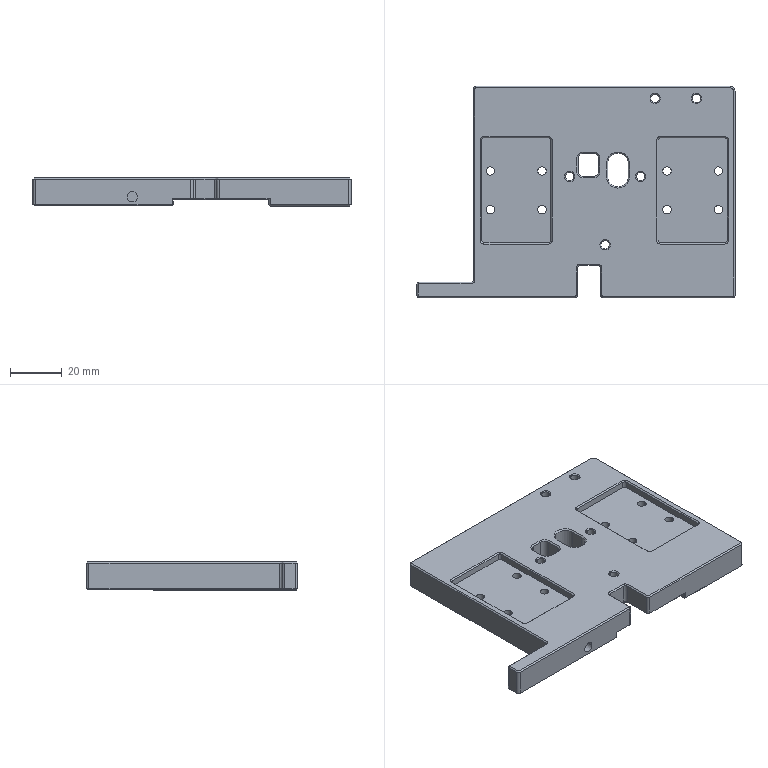NC program | NX | posted with a generic post | part box 123.41 x 82 x 11.078 mm
Whole program:
N10 G17 G21 G94 G90
(ZLEVEL_PROFILE_COPY_COPY_COPY_COPY_COPY_1 , TOOL : D10)
N12 T10 M6
N14 G54
N16 G17 G0 G90 X-32.118 Y-47.254 S9500 M3
N18 G43 Z30. H10
N20 Z4.5
N22 G94 G1 Z3. F1000.
N24 X-32.353 Y-46.848
N26 G3 X-33.219 Y-46.348 R1.
N28 G1 X-38.699 F1200.
N30 X-38.713 Y-46.35
N32 G2 X-45.055 Y-39.992 R6.351
N34 G1 Y29.65
N36 X-60.709
N38 G2 X-62.088 Y29.803 R6.346
N40 G1 X-62.403 Y29.887
N42 G2 X-63.961 Y30.555 R5.799
N44 G1 X-64.243 Y30.729
N46 G2 X-67.055 Y36.009 R6.347
N48 G1 Y39.985
N50 G2 X-66.732 Y41.879 R5.928
N52 X-63.518 Y45.645 R6.354
N54 X-60.764 Y46.31 R6.48
N56 X-55.255 Y46.345 R551.466
N58 G3 X-54.389 Y46.846 R1.
N60 G1 X-54.152 Y47.257
N62 Z4.5
N64 G0 Z30.
N66 X-54.149 Y47.258
N68 Z3.5
N70 G1 Z2. F1000.
N72 X-54.388 Y46.846
N74 G2 X-55.255 Y46.346 R1.
N76 G3 X-60.764 Y46.311 R383.966 F1200.
N78 X-63.977 Y45.394 R6.459
N80 X-65.035 Y44.59 R7.973
N82 X-66.754 Y41.818 R6.483
N84 X-67.055 Y39.985 R5.907
N86 G1 Y36.009
N88 G3 X-64.243 Y30.729 R6.348
N90 G1 X-63.961 Y30.555
N92 G3 X-62.403 Y29.887 R5.803
N94 G1 X-62.088 Y29.803
N96 G3 X-60.709 Y29.65 R6.348
N98 G1 X-45.055
N100 Y-39.992
N102 G3 X-38.713 Y-46.35 R6.351
N104 G1 X-38.699 Y-46.348
N106 X-33.219
N108 G2 X-32.353 Y-46.848 R1.
N110 G1 X-32.118 Y-47.255
N112 Z3.5
N114 G0 Z30.
N116 Z2.5
N118 G1 Z1. F1000.
N120 X-32.353 Y-46.848
N122 G3 X-33.219 Y-46.348 R1.
N124 G1 X-38.699 F1200.
N126 X-38.713 Y-46.35
N128 G2 X-45.055 Y-39.992 R6.351
N130 G1 Y29.65
N132 X-60.709
N134 G2 X-62.089 Y29.803 R6.35
N136 G1 X-62.402 Y29.886
N138 G2 X-63.962 Y30.556 R5.808
N140 G1 X-64.243 Y30.729
N142 G2 X-67.055 Y36.009 R6.348
N144 G1 Y39.985
N146 G2 X-63.977 Y45.4 R6.458
N148 X-60.764 Y46.315 R6.42
N150 X-55.255 Y46.348 R309.642
N152 G3 X-54.387 Y46.845 R1.
N154 G1 X-54.146 Y47.259
N156 Z2.5
N158 G0 Z30.
N160 X-54.153 Y47.261
N162 Z1.5
N164 G1 Z0. F1000.
N166 X-54.39 Y46.849
N168 G2 X-55.255 Y46.348 R1.
N170 G1 X-60.764 Y46.336 F1200.
N172 G3 X-63.518 Y45.676 R6.465
N174 X-67.055 Y39.985 R6.391
N176 G1 Y36.009
N178 G3 X-64.243 Y30.729 R6.348
N180 G1 X-63.962 Y30.556
N182 G3 X-62.402 Y29.886 R5.812
N184 G1 X-62.089 Y29.803
N186 G3 X-60.709 Y29.65 R6.364
N188 G1 X-45.055
N190 Y-39.992
N192 G3 X-38.713 Y-46.35 R6.351
N194 G1 X-38.699 Y-46.348
N196 X-33.219
N198 G2 X-32.353 Y-46.848 R1.
N200 G1 X-32.118 Y-47.255
N202 Z1.5
N204 G0 Z30.
N206 X-32.063 Y-47.35
N208 Z0.5
N210 G1 Z-1. F1000.
N212 X-32.353 Y-46.848
N214 G3 X-33.219 Y-46.348 R1.
N216 G1 X-38.269 F1200.
N218 X-38.705 Y-46.35
N220 G2 X-45.055 Y-40. R6.35
N222 G1 Y29.65
N224 X-60.701
N226 G2 X-67.055 Y36. R6.35
N228 G1 Y40.
N230 G2 X-60.764 Y46.346 R6.355
N232 G1 X-60.305 Y46.348
N234 X-55.255
N236 G3 X-54.389 Y46.848 R1.
N238 G1 X-54.099 Y47.35
N240 Z0.5
N242 G0 Z30.
N244 M5
(FLOOR_WALL_COPY , TOOL : D63)
N246 T01 M6
N248 G54
N250 G17 G0 G90 X96.205 Y-40.997 S6500 M3
N252 G43 Z30. H1
N254 Z6.
N256 G94 G1 Z3. F1250.
N258 X93.205
N260 X-93.205
N262 Y-12.599
N264 X93.205
N266 Y15.8
N268 X-93.205
N270 X-96.205
N272 Z6.
N274 G0 Z30.
N276 X96.205 Y-40.998
N278 Z5.
N280 G1 Z2.
N282 X93.205
N284 X-93.205
N286 Y-12.599
N288 X93.205
N290 Y15.8
N292 X-93.205
N294 X-96.205
N296 Z5.
N298 G0 Z30.
N300 X96.205 Y-40.998
N302 Z4.
N304 G1 Z1.
N306 X93.205
N308 X-93.205
N310 Y-12.599
N312 X93.205
N314 Y15.8
N316 X-93.205
N318 X-96.205
N320 Z4.
N322 G0 Z30.
N324 X96.205 Y-40.998
N326 Z3.
N328 G1 Z0.
N330 X93.205
N332 X-93.205
N334 Y-12.599
N336 X93.205
N338 Y15.8
N340 X-93.205
N342 X-96.205
N344 Z3.
N346 G0 Z30.
N348 M5
(FLOOR_WALL_1_COPY , TOOL : D4)
N350 T04 M6
N352 G54
N354 G17 G0 G90 X-39.538 Y-43.919 S9500 M3
N356 G43 Z30. H4
N358 Z1.389
N360 G94 G1 Z-0.111 F1000.
N362 X-38.548 Y-42.888
N364 G3 X-38.452 Y-42.5 R0.4
N366 G1 X-62.75 Y41.438
N368 G2 X-61.009 Y42.481 R2.5
N370 G1 X-36.41 Y-42.5
N372 X-34.367
N374 X-58.972 Y42.5
N376 X-56.93
N378 X-32.324 Y-42.5
N380 X-30.282
N382 X-54.887 Y42.5
N384 X-52.844
N386 X-28.239 Y-42.5
N388 X-26.197
N390 X-50.802 Y42.5
N392 X-48.759
N394 X-24.154 Y-42.5
N396 X-22.111
N398 X-46.716 Y42.5
N400 X-44.674
N402 X-20.069 Y-42.5
N404 X-18.026
N406 X-42.631 Y42.5
N408 X-40.589
N410 X-15.983 Y-42.5
N412 X-13.941
N414 X-38.546 Y42.5
N416 X-36.503
N418 X-11.898 Y-42.5
N420 X-9.856
N422 X-34.461 Y42.5
N424 X-32.418
N426 X-7.813 Y-42.5
N428 X-5.77
N430 X-30.376 Y42.5
N432 X-28.333
N434 X-5.705 Y-35.67
N436 Y-28.614
N438 X-26.29 Y42.5
N440 X-24.248
N442 X-5.705 Y-21.558
N444 Y-14.501
N446 X-22.205 Y42.5
N448 X-20.162
N450 X-5.705 Y-7.445
N452 Y-0.389
N454 X-18.12 Y42.5
N456 X-16.077
N458 X-5.705 Y6.668
N460 Y13.724
N462 X-14.035 Y42.5
N464 X-11.992
N466 X-5.705 Y20.78
N468 Y27.837
N470 X-9.949 Y42.5
N472 G3 X-10.238 Y42.777 R0.4
N474 G1 Y44.
N476 Z1.389
N478 G0 Z30.
N480 X63.897 Y-41.807
N482 Z-2.422
N484 G1 Z-3.922
N486 X63.257 Y-40.697
N488 G3 X62.91 Y-40.497 R0.4
N490 G1 X28.816
N492 G3 X28.855 Y-40. R3.2
N494 G1 Y-38.585
N496 X63.206
N498 X63.205 Y-36.673
N500 X28.855
N502 Y-34.761
N504 X63.205
N506 Y-32.849
N508 X28.855
N510 Y-30.937
N512 X63.205
N514 Y-29.026
N516 X28.855
N518 Y-27.114
N520 X63.205
N522 Y-25.202
N524 X28.855
N526 Y-23.29
N528 X63.205
N530 Y-21.378
N532 X28.855
N534 Y-19.466
N536 X63.205
N538 Y-17.554
N540 X61.205
N542 G3 X60.858 Y-17.754 R0.4
N544 G1 X64.705
N546 Z-2.422
N548 G0 Z30.
N550 X64.895 Y-16.033
N552 Z-2.422
N554 G1 Z-3.922
N556 X63.536 Y-15.924
N558 G3 X63.175 Y-16.096 R0.4
N560 G2 X60.705 Y-17.393 R3.
N562 G1 X28.655
N564 Y-40.
N566 G2 X27.357 Y-42.47 R3.
N568 G3 X27.186 Y-42.831 R0.4
N570 G1 X27.295 Y-44.191
N572 Z-2.422
N574 G0 Z30.
(ZLEVEL_PROFILE_1_COPY_1_COPY_COPY_COPY , TOOL : D4A45)
N576 T02 M6
N578 G17 G43 G0 G90 X33.968 Y-8.586 Z30. S9500 H2 M3
N580 Z-0.1
N582 G94 G1 Z-1.1 F1000.
N584 X33.348 Y-8.794
N586 G3 X33.364 Y-9.194 R0.4
N588 G1 X33.515 Y-9.432
N590 G3 X35.345 Y-5.964 R-2.185
N592 X33.166 Y-7.607 R2.184
N594 X33.364 Y-9.194 R2.17
N596 X33.706 Y-9.401 R0.4
N598 G1 X34.746 Y-9.424
N600 Z-0.1
N602 G0 Z30.
N604 X53.968 Y-8.586
N606 Z-0.1
N608 G1 Z-1.1
N610 X53.348 Y-8.794
N612 G3 X53.364 Y-9.194 R0.4
N614 G1 X53.519 Y-9.438
N616 G3 X55.019 Y-5.979 R-2.185
N618 X53.166 Y-7.607 R2.182
N620 X53.364 Y-9.194 R2.17
N622 X53.706 Y-9.401 R0.4
N624 G1 X54.743 Y-9.424
N626 Z-0.1
N628 G0 Z30.
N630 X34.743 Y8.128
N632 Z-0.1
N634 G1 Z-1.1
N636 X34.488 Y8.736
N638 G3 X34.091 Y8.685 R0.4
N640 G1 X33.836 Y8.489
N642 G3 X35.334 Y9.037 R-2.185
N644 X34.695 Y8.956 R2.17
N646 X34.091 Y8.685 R2.142
N648 X33.911 Y8.328 R0.4
N650 G1 X33.967 Y7.285
N652 Z-0.1
N654 G0 Z30.
N656 X55.562 Y8.208
N658 Z-0.1
N660 G1 Z-1.1
N662 X55.695 Y8.853
N664 G3 X55.339 Y9.036 R0.4
N666 G1 X55.019 Y9.02
N668 X54.753 Y8.972
N670 X54.695 Y8.956
N672 G3 X53.835 Y8.489 R2.105
N674 X53.42 Y7.992 R2.096
N676 X55.339 Y9.036 R-2.185
N678 X54.988 Y8.845 R0.4
N680 G1 X54.443 Y7.955
N682 Z-0.1
N684 G0 Z30.
N686 X-14.06 Y-9.385
N688 Z-0.1
N690 G1 Z-1.1
N692 X-13.564 Y-10.245
N694 G3 X-13.217 Y-10.445 R0.4
N696 X-14.969 Y-6.665 R-2.296
N698 X-14.583 Y-9.994 R2.295
N700 X-13.217 Y-10.445 R2.296
N702 X-12.871 Y-10.245 R0.4
N704 G1 X-12.374 Y-9.385
N706 Z-0.1
N708 G0 Z30.
N710 X-34.454 Y7.694
N712 Z-0.1
N714 G1 Z-1.1
N716 X-35.313 Y7.198
N718 G3 X-35.513 Y6.851 R0.4
N720 X-34.15 Y8.949 R-2.296
N722 X-35.5 Y7.098 R2.292
N724 X-35.513 Y6.851 R2.296
N726 X-35.313 Y6.505 R0.4
N728 G1 X-34.453 Y6.008
N730 Z-0.1
N732 G0 Z30.
N734 X-12.374 Y8.087
N736 Z-0.1
N738 G1 Z-1.1
N740 X-12.871 Y8.947
N742 G3 X-13.218 Y9.147 R0.4
N744 X-14.15 Y8.949 R2.296
N746 X-15.5 Y7.098 R2.292
N748 X-13.218 Y9.147 R-2.296
N750 X-13.564 Y8.947 R0.4
N752 G1 X-14.06 Y8.087
N754 Z-0.1
N756 G0 Z30.
N758 X-34.702 Y-7.972
N760 Z-0.1
N762 G1 Z-1.1
N764 X-34.98 Y-9.382
N766 G3 X-34.851 Y-9.761 R0.4
N768 G1 X-34.582 Y-9.995
N770 X-34.301 Y-10.172
N772 G3 X-34.851 Y-9.761 R-2.296
N774 X-34.465 Y-9.867 R0.4
N776 G1 X-33.504 Y-9.616
N778 Z-0.1
N780 G0 Z30.
N782 X-6.063 Y41.097
N784 Z-0.1
N786 G1 Z-1.1
N788 X-6.557 Y40.812
N790 G3 X-6.757 Y40.465 R0.4
N792 G1 Y-40.522
N794 G2 X-7.703 Y-41.448 R0.951
N796 G1 X-38.704
N798 G2 X-40.153 Y-39.999 R1.448
N800 G1 Y34.
N802 G3 X-40.705 Y34.552 R0.552
N804 G1 X-60.697
N806 G2 X-62.153 Y36.007 R1.455
N808 G1 Y39.867
N810 X-62.151 Y40.025
N812 G2 X-60.711 Y41.448 R1.44
N814 G1 X-7.704
N816 G2 X-6.757 Y40.465 R0.952
N818 G3 X-6.568 Y40.113 R0.4
N820 G1 X-5.957 Y39.734
N822 Z-0.1
N824 G0 Z30.
N826 X62.974 Y40.646
N828 Z-0.1
N830 G1 Z-1.1
N832 X62.463 Y40.351
N834 G3 X62.263 Y40.004 R0.4
N836 G1 Y-14.39
N838 G2 X60.705 Y-15.952 R1.566
N840 G1 X30.291
N842 G2 X29.237 Y-14.898 R1.054
N844 G1 Y40.465
N846 G2 X30.295 Y41.559 R1.063
N848 G1 X60.709
N850 G2 X62.263 Y40.004 R1.554
N852 G3 X62.463 Y39.658 R0.4
N854 G1 X63.063 Y39.312
N856 Z-0.1
N858 G0 Z30.
(ZLEVEL_PROFILE_1_COPY_1_COPY_COPY_COPY_COPY_COPY , TOOL : D4A45)
N860 Z30.
N862 X30.616 Y-36.517
N864 Z-3.922
N866 G1 Z-4.922
N868 X30.359 Y-37.135
N870 G3 X30.706 Y-37.335 R0.4
N872 X31.738 Y-36.302 R1.033
N874 X30.706 Y-37.335 R-1.033
N876 X31.052 Y-37.135 R0.4
N878 G1 X30.795 Y-36.517
N880 Z-3.922
N882 G0 Z30.
N884 X46.616
N886 Z-3.922
N888 G1 Z-4.922
N890 X46.36 Y-37.135
N892 G3 X46.706 Y-37.335 R0.4
N894 X47.74 Y-36.301 R1.034
N896 X46.706 Y-37.335 R-1.034
N898 X47.053 Y-37.135 R0.4
N900 G1 X46.796 Y-36.517
N902 Z-3.922
N904 G0 Z30.
N906 X62.963 Y-17.355
N908 Z-3.922
N910 G1 Z-4.922
N912 X62.263 Y-17.073
N914 G3 X62.163 Y-17.246 R0.2
N916 G1 X62.164 Y-38.726
N918 X62.161 Y-39.017
N920 G2 X59.702 Y-41.459 R2.459
N922 G1 X28.51
N924 G3 X28.337 Y-41.559 R0.2
N926 G1 X28.56 Y-42.259
N928 Z-3.922
N930 G0 Z30.
N932 M5
(刀补4 , TOOL : D4)
N934 T04 M6
N936 G54
N938 G17 G0 G90 X26.151 Y-16.196 S9500 M3
N940 G43 Z30. H4
N942 Z-1.
N944 G94 G1 Z-2.5 F1000.
N946 G41 X26.245 Y-16.162 D4
N948 X27.545 Y-15.411
N950 G3 X27.745 Y-15.065 R0.4
N952 G1 Y40.5
N954 G3 X27.545 Y40.846 R0.4
N956 G1 X26.245 Y41.597
N958 G40
N960 X26.151 Y41.631
N962 Z-1.
N964 G0 Z30.
N966 X-3.561
N968 Z-1.
N970 G1 Z-2.5
N972 G41 X-3.655 Y41.597
N974 X-4.955 Y40.846
N976 G3 X-5.155 Y40.5 R0.4
N978 G1 Y-40.5
N980 G3 X-4.955 Y-40.846 R0.4
N982 G1 X-3.655 Y-41.597
N984 G40
N986 X-3.561 Y-41.631
N988 Z-1.
N990 G0 Z30.
N992 M5
N994 M2